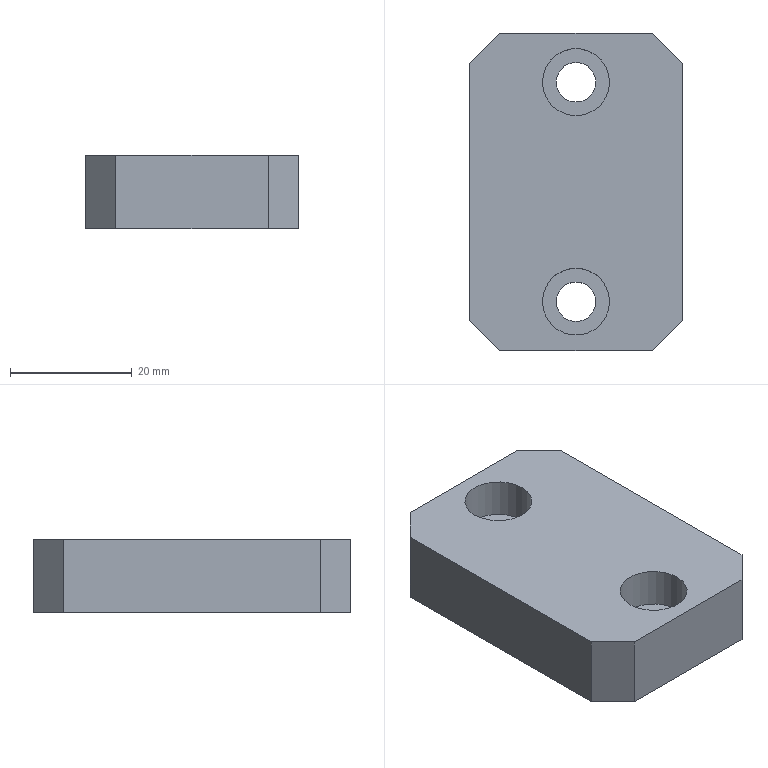Part | STEP file | lll_id314_x_t | 1 solid | 16 faces | box 35 x 52 x 12 mm | volume 19640 mm3 | plane 12 | cylinder 4 | commonest cylinder face diameters 6.5 x2 11 x2
STEP:
#1=CARTESIAN_POINT('',(76.553,9.,100.5));
#2=VERTEX_POINT('',#1);
#3=CARTESIAN_POINT('',(51.553,9.,100.5));
#4=VERTEX_POINT('',#3);
#5=CARTESIAN_POINT('',(-312.69,9.,100.5));
#6=DIRECTION('',(-1.,0.,0.));
#7=VECTOR('',#6,1.);
#8=LINE('',#5,#7);
#9=EDGE_CURVE('',#2,#4,#8,.T.);
#10=ORIENTED_EDGE('',*,*,#9,.T.);
#11=CARTESIAN_POINT('',(51.553,9.,88.5));
#12=VERTEX_POINT('',#11);
#13=CARTESIAN_POINT('',(51.553,9.,110.5));
#14=DIRECTION('',(0.,0.,1.));
#15=VECTOR('',#14,1.);
#16=LINE('',#13,#15);
#17=EDGE_CURVE('',#12,#4,#16,.T.);
#18=ORIENTED_EDGE('',*,*,#17,.F.);
#19=CARTESIAN_POINT('',(76.553,9.,88.5));
#20=VERTEX_POINT('',#19);
#21=CARTESIAN_POINT('',(64.053,9.,88.5));
#22=DIRECTION('',(1.,0.,0.));
#23=VECTOR('',#22,1.);
#24=LINE('',#21,#23);
#25=EDGE_CURVE('',#12,#20,#24,.T.);
#26=ORIENTED_EDGE('',*,*,#25,.T.);
#27=CARTESIAN_POINT('',(76.553,9.,88.5));
#28=DIRECTION('',(0.,0.,-1.));
#29=VECTOR('',#28,1.);
#30=LINE('',#27,#29);
#31=EDGE_CURVE('',#2,#20,#30,.T.);
#32=ORIENTED_EDGE('',*,*,#31,.F.);
#33=EDGE_LOOP('',(#10,#18,#26,#32));
#34=FACE_OUTER_BOUND('',#33,.T.);
#35=CARTESIAN_POINT('',(47.219,9.,110.5));
#36=DIRECTION('',(0.,-1.,0.));
#37=DIRECTION('',(0.,0.,1.));
#38=AXIS2_PLACEMENT_3D('',#35,#36,#37);
#39=PLANE('',#38);
#40=ADVANCED_FACE('',(#34),#39,.T.);
#41=CARTESIAN_POINT('',(81.553,56.,88.5));
#42=VERTEX_POINT('',#41);
#43=CARTESIAN_POINT('',(81.553,14.,88.5));
#44=VERTEX_POINT('',#43);
#45=CARTESIAN_POINT('',(81.553,34.,88.5));
#46=DIRECTION('',(0.,-1.,0.));
#47=VECTOR('',#46,1.);
#48=LINE('',#45,#47);
#49=EDGE_CURVE('',#42,#44,#48,.T.);
#50=ORIENTED_EDGE('',*,*,#49,.T.);
#51=CARTESIAN_POINT('',(86.803,19.25,88.5));
#52=DIRECTION('',(0.7071,0.7071,0.));
#53=VECTOR('',#52,1.);
#54=LINE('',#51,#53);
#55=EDGE_CURVE('',#20,#44,#54,.T.);
#56=ORIENTED_EDGE('',*,*,#55,.F.);
#57=ORIENTED_EDGE('',*,*,#25,.F.);
#58=CARTESIAN_POINT('',(46.553,14.,88.5));
#59=VERTEX_POINT('',#58);
#60=CARTESIAN_POINT('',(41.303,19.25,88.5));
#61=DIRECTION('',(0.7071,-0.7071,0.));
#62=VECTOR('',#61,1.);
#63=LINE('',#60,#62);
#64=EDGE_CURVE('',#59,#12,#63,.T.);
#65=ORIENTED_EDGE('',*,*,#64,.F.);
#66=CARTESIAN_POINT('',(46.553,56.,88.5));
#67=VERTEX_POINT('',#66);
#68=CARTESIAN_POINT('',(46.553,34.,88.5));
#69=DIRECTION('',(0.,-1.,0.));
#70=VECTOR('',#69,1.);
#71=LINE('',#68,#70);
#72=EDGE_CURVE('',#67,#59,#71,.T.);
#73=ORIENTED_EDGE('',*,*,#72,.F.);
#74=CARTESIAN_POINT('',(51.553,61.,88.5));
#75=VERTEX_POINT('',#74);
#76=CARTESIAN_POINT('',(44.303,53.75,88.5));
#77=DIRECTION('',(-0.7071,-0.7071,0.));
#78=VECTOR('',#77,1.);
#79=LINE('',#76,#78);
#80=EDGE_CURVE('',#75,#67,#79,.T.);
#81=ORIENTED_EDGE('',*,*,#80,.F.);
#82=CARTESIAN_POINT('',(76.553,61.,88.5));
#83=VERTEX_POINT('',#82);
#84=CARTESIAN_POINT('',(64.053,61.,88.5));
#85=DIRECTION('',(1.,0.,0.));
#86=VECTOR('',#85,1.);
#87=LINE('',#84,#86);
#88=EDGE_CURVE('',#75,#83,#87,.T.);
#89=ORIENTED_EDGE('',*,*,#88,.T.);
#90=CARTESIAN_POINT('',(83.803,53.75,88.5));
#91=DIRECTION('',(-0.7071,0.7071,0.));
#92=VECTOR('',#91,1.);
#93=LINE('',#90,#92);
#94=EDGE_CURVE('',#42,#83,#93,.T.);
#95=ORIENTED_EDGE('',*,*,#94,.F.);
#96=EDGE_LOOP('',(#50,#56,#57,#65,#73,#81,#89,#95));
#97=FACE_BOUND('',#96,.T.);
#98=CARTESIAN_POINT('',(67.303,17.,88.5));
#99=VERTEX_POINT('',#98);
#100=CARTESIAN_POINT('',(64.053,17.,88.5));
#101=DIRECTION('',(0.,0.,1.));
#102=DIRECTION('',(1.,0.,0.));
#103=AXIS2_PLACEMENT_3D('',#100,#101,#102);
#104=CIRCLE('',#103,3.25);
#105=EDGE_CURVE('',#99,#99,#104,.T.);
#106=ORIENTED_EDGE('',*,*,#105,.T.);
#107=EDGE_LOOP('',(#106));
#108=FACE_BOUND('',#107,.T.);
#109=CARTESIAN_POINT('',(67.303,53.,88.5));
#110=VERTEX_POINT('',#109);
#111=CARTESIAN_POINT('',(64.053,53.,88.5));
#112=DIRECTION('',(0.,0.,1.));
#113=DIRECTION('',(1.,0.,0.));
#114=AXIS2_PLACEMENT_3D('',#111,#112,#113);
#115=CIRCLE('',#114,3.25);
#116=EDGE_CURVE('',#110,#110,#115,.T.);
#117=ORIENTED_EDGE('',*,*,#116,.T.);
#118=EDGE_LOOP('',(#117));
#119=FACE_BOUND('',#118,.T.);
#120=CARTESIAN_POINT('',(64.053,34.,88.5));
#121=DIRECTION('',(0.,0.,-1.));
#122=DIRECTION('',(-1.,0.,0.));
#123=AXIS2_PLACEMENT_3D('',#120,#121,#122);
#124=PLANE('',#123);
#125=ADVANCED_FACE('',(#97,#108,#119),#124,.T.);
#126=CARTESIAN_POINT('',(76.553,61.,100.5));
#127=VERTEX_POINT('',#126);
#128=CARTESIAN_POINT('',(51.553,61.,100.5));
#129=VERTEX_POINT('',#128);
#130=CARTESIAN_POINT('',(-312.69,61.,100.5));
#131=DIRECTION('',(-1.,0.,0.));
#132=VECTOR('',#131,1.);
#133=LINE('',#130,#132);
#134=EDGE_CURVE('',#127,#129,#133,.T.);
#135=ORIENTED_EDGE('',*,*,#134,.T.);
#136=CARTESIAN_POINT('',(46.553,56.,100.5));
#137=VERTEX_POINT('',#136);
#138=CARTESIAN_POINT('',(-222.363,-212.917,100.5));
#139=DIRECTION('',(0.7071,0.7071,0.));
#140=VECTOR('',#139,1.);
#141=LINE('',#138,#140);
#142=EDGE_CURVE('',#137,#129,#141,.T.);
#143=ORIENTED_EDGE('',*,*,#142,.F.);
#144=CARTESIAN_POINT('',(46.553,14.,100.5));
#145=VERTEX_POINT('',#144);
#146=CARTESIAN_POINT('',(46.553,-122.59,100.5));
#147=DIRECTION('',(0.,1.,0.));
#148=VECTOR('',#147,1.);
#149=LINE('',#146,#148);
#150=EDGE_CURVE('',#145,#137,#149,.T.);
#151=ORIENTED_EDGE('',*,*,#150,.F.);
#152=CARTESIAN_POINT('',(-68.773,129.327,100.5));
#153=DIRECTION('',(-0.7071,0.7071,0.));
#154=VECTOR('',#153,1.);
#155=LINE('',#152,#154);
#156=EDGE_CURVE('',#4,#145,#155,.T.);
#157=ORIENTED_EDGE('',*,*,#156,.F.);
#158=ORIENTED_EDGE('',*,*,#9,.F.);
#159=CARTESIAN_POINT('',(81.553,14.,100.5));
#160=VERTEX_POINT('',#159);
#161=CARTESIAN_POINT('',(-179.863,-247.417,100.5));
#162=DIRECTION('',(-0.7071,-0.7071,0.));
#163=VECTOR('',#162,1.);
#164=LINE('',#161,#163);
#165=EDGE_CURVE('',#160,#2,#164,.T.);
#166=ORIENTED_EDGE('',*,*,#165,.F.);
#167=CARTESIAN_POINT('',(81.553,56.,100.5));
#168=VERTEX_POINT('',#167);
#169=CARTESIAN_POINT('',(81.553,-122.59,100.5));
#170=DIRECTION('',(0.,1.,0.));
#171=VECTOR('',#170,1.);
#172=LINE('',#169,#171);
#173=EDGE_CURVE('',#160,#168,#172,.T.);
#174=ORIENTED_EDGE('',*,*,#173,.T.);
#175=CARTESIAN_POINT('',(-26.273,163.827,100.5));
#176=DIRECTION('',(0.7071,-0.7071,0.));
#177=VECTOR('',#176,1.);
#178=LINE('',#175,#177);
#179=EDGE_CURVE('',#127,#168,#178,.T.);
#180=ORIENTED_EDGE('',*,*,#179,.F.);
#181=EDGE_LOOP('',(#135,#143,#151,#157,#158,#166,#174,#180));
#182=FACE_BOUND('',#181,.T.);
#183=CARTESIAN_POINT('',(58.553,17.,100.5));
#184=VERTEX_POINT('',#183);
#185=CARTESIAN_POINT('',(64.053,17.,100.5));
#186=DIRECTION('',(0.,0.,1.));
#187=DIRECTION('',(-1.,0.,0.));
#188=AXIS2_PLACEMENT_3D('',#185,#186,#187);
#189=CIRCLE('',#188,5.5);
#190=EDGE_CURVE('',#184,#184,#189,.T.);
#191=ORIENTED_EDGE('',*,*,#190,.F.);
#192=EDGE_LOOP('',(#191));
#193=FACE_BOUND('',#192,.T.);
#194=CARTESIAN_POINT('',(58.553,53.,100.5));
#195=VERTEX_POINT('',#194);
#196=CARTESIAN_POINT('',(64.053,53.,100.5));
#197=DIRECTION('',(0.,0.,-1.));
#198=DIRECTION('',(-1.,0.,0.));
#199=AXIS2_PLACEMENT_3D('',#196,#197,#198);
#200=CIRCLE('',#199,5.5);
#201=EDGE_CURVE('',#195,#195,#200,.T.);
#202=ORIENTED_EDGE('',*,*,#201,.T.);
#203=EDGE_LOOP('',(#202));
#204=FACE_BOUND('',#203,.T.);
#205=CARTESIAN_POINT('',(-312.69,-122.59,100.5));
#206=DIRECTION('',(0.,0.,-1.));
#207=DIRECTION('',(0.,-1.,0.));
#208=AXIS2_PLACEMENT_3D('',#205,#206,#207);
#209=PLANE('',#208);
#210=ADVANCED_FACE('',(#182,#193,#204),#209,.F.);
#211=ORIENTED_EDGE('',*,*,#88,.F.);
#212=CARTESIAN_POINT('',(51.553,61.,88.5));
#213=DIRECTION('',(0.,0.,-1.));
#214=VECTOR('',#213,1.);
#215=LINE('',#212,#214);
#216=EDGE_CURVE('',#129,#75,#215,.T.);
#217=ORIENTED_EDGE('',*,*,#216,.F.);
#218=ORIENTED_EDGE('',*,*,#134,.F.);
#219=CARTESIAN_POINT('',(76.553,61.,110.5));
#220=DIRECTION('',(0.,0.,1.));
#221=VECTOR('',#220,1.);
#222=LINE('',#219,#221);
#223=EDGE_CURVE('',#83,#127,#222,.T.);
#224=ORIENTED_EDGE('',*,*,#223,.F.);
#225=EDGE_LOOP('',(#211,#217,#218,#224));
#226=FACE_OUTER_BOUND('',#225,.T.);
#227=CARTESIAN_POINT('',(47.219,61.,110.5));
#228=DIRECTION('',(0.,-1.,0.));
#229=DIRECTION('',(0.,0.,1.));
#230=AXIS2_PLACEMENT_3D('',#227,#228,#229);
#231=PLANE('',#230);
#232=ADVANCED_FACE('',(#226),#231,.F.);
#233=ORIENTED_EDGE('',*,*,#105,.F.);
#234=EDGE_LOOP('',(#233));
#235=FACE_BOUND('',#234,.T.);
#236=CARTESIAN_POINT('',(60.803,17.,94.));
#237=VERTEX_POINT('',#236);
#238=CARTESIAN_POINT('',(64.053,17.,94.));
#239=DIRECTION('',(0.,0.,1.));
#240=DIRECTION('',(-1.,0.,0.));
#241=AXIS2_PLACEMENT_3D('',#238,#239,#240);
#242=CIRCLE('',#241,3.25);
#243=EDGE_CURVE('',#237,#237,#242,.T.);
#244=ORIENTED_EDGE('',*,*,#243,.T.);
#245=EDGE_LOOP('',(#244));
#246=FACE_BOUND('',#245,.T.);
#247=CARTESIAN_POINT('',(64.053,17.,-199.5));
#248=DIRECTION('',(0.,0.,-1.));
#249=DIRECTION('',(-1.,0.,0.));
#250=AXIS2_PLACEMENT_3D('',#247,#248,#249);
#251=CYLINDRICAL_SURFACE('',#250,3.25);
#252=ADVANCED_FACE('',(#235,#246),#251,.F.);
#253=ORIENTED_EDGE('',*,*,#243,.F.);
#254=EDGE_LOOP('',(#253));
#255=FACE_BOUND('',#254,.T.);
#256=CARTESIAN_POINT('',(58.553,17.,94.));
#257=VERTEX_POINT('',#256);
#258=CARTESIAN_POINT('',(64.053,17.,94.));
#259=DIRECTION('',(0.,0.,1.));
#260=DIRECTION('',(-1.,0.,0.));
#261=AXIS2_PLACEMENT_3D('',#258,#259,#260);
#262=CIRCLE('',#261,5.5);
#263=EDGE_CURVE('',#257,#257,#262,.T.);
#264=ORIENTED_EDGE('',*,*,#263,.T.);
#265=EDGE_LOOP('',(#264));
#266=FACE_BOUND('',#265,.T.);
#267=CARTESIAN_POINT('',(64.053,17.,94.));
#268=DIRECTION('',(0.,0.,-1.));
#269=DIRECTION('',(-1.,0.,0.));
#270=AXIS2_PLACEMENT_3D('',#267,#268,#269);
#271=PLANE('',#270);
#272=ADVANCED_FACE('',(#255,#266),#271,.F.);
#273=ORIENTED_EDGE('',*,*,#263,.F.);
#274=EDGE_LOOP('',(#273));
#275=FACE_BOUND('',#274,.T.);
#276=ORIENTED_EDGE('',*,*,#190,.T.);
#277=EDGE_LOOP('',(#276));
#278=FACE_BOUND('',#277,.T.);
#279=CARTESIAN_POINT('',(64.053,17.,100.5));
#280=DIRECTION('',(0.,0.,-1.));
#281=DIRECTION('',(-1.,0.,0.));
#282=AXIS2_PLACEMENT_3D('',#279,#280,#281);
#283=CYLINDRICAL_SURFACE('',#282,5.5);
#284=ADVANCED_FACE('',(#275,#278),#283,.F.);
#285=ORIENTED_EDGE('',*,*,#116,.F.);
#286=EDGE_LOOP('',(#285));
#287=FACE_BOUND('',#286,.T.);
#288=CARTESIAN_POINT('',(60.803,53.,94.));
#289=VERTEX_POINT('',#288);
#290=CARTESIAN_POINT('',(64.053,53.,94.));
#291=DIRECTION('',(0.,0.,-1.));
#292=DIRECTION('',(-1.,0.,0.));
#293=AXIS2_PLACEMENT_3D('',#290,#291,#292);
#294=CIRCLE('',#293,3.25);
#295=EDGE_CURVE('',#289,#289,#294,.T.);
#296=ORIENTED_EDGE('',*,*,#295,.F.);
#297=EDGE_LOOP('',(#296));
#298=FACE_BOUND('',#297,.T.);
#299=CARTESIAN_POINT('',(64.053,53.,-199.5));
#300=DIRECTION('',(0.,0.,-1.));
#301=DIRECTION('',(-1.,0.,0.));
#302=AXIS2_PLACEMENT_3D('',#299,#300,#301);
#303=CYLINDRICAL_SURFACE('',#302,3.25);
#304=ADVANCED_FACE('',(#287,#298),#303,.F.);
#305=ORIENTED_EDGE('',*,*,#295,.T.);
#306=EDGE_LOOP('',(#305));
#307=FACE_BOUND('',#306,.T.);
#308=CARTESIAN_POINT('',(58.553,53.,94.));
#309=VERTEX_POINT('',#308);
#310=CARTESIAN_POINT('',(64.053,53.,94.));
#311=DIRECTION('',(0.,0.,-1.));
#312=DIRECTION('',(-1.,0.,0.));
#313=AXIS2_PLACEMENT_3D('',#310,#311,#312);
#314=CIRCLE('',#313,5.5);
#315=EDGE_CURVE('',#309,#309,#314,.T.);
#316=ORIENTED_EDGE('',*,*,#315,.F.);
#317=EDGE_LOOP('',(#316));
#318=FACE_BOUND('',#317,.T.);
#319=CARTESIAN_POINT('',(64.053,53.,94.));
#320=DIRECTION('',(0.,0.,-1.));
#321=DIRECTION('',(-1.,0.,0.));
#322=AXIS2_PLACEMENT_3D('',#319,#320,#321);
#323=PLANE('',#322);
#324=ADVANCED_FACE('',(#307,#318),#323,.F.);
#325=ORIENTED_EDGE('',*,*,#315,.T.);
#326=EDGE_LOOP('',(#325));
#327=FACE_BOUND('',#326,.T.);
#328=ORIENTED_EDGE('',*,*,#201,.F.);
#329=EDGE_LOOP('',(#328));
#330=FACE_BOUND('',#329,.T.);
#331=CARTESIAN_POINT('',(64.053,53.,100.5));
#332=DIRECTION('',(0.,0.,-1.));
#333=DIRECTION('',(-1.,0.,0.));
#334=AXIS2_PLACEMENT_3D('',#331,#332,#333);
#335=CYLINDRICAL_SURFACE('',#334,5.5);
#336=ADVANCED_FACE('',(#327,#330),#335,.F.);
#337=ORIENTED_EDGE('',*,*,#72,.T.);
#338=CARTESIAN_POINT('',(46.553,14.,100.5));
#339=DIRECTION('',(0.,0.,-1.));
#340=VECTOR('',#339,1.);
#341=LINE('',#338,#340);
#342=EDGE_CURVE('',#145,#59,#341,.T.);
#343=ORIENTED_EDGE('',*,*,#342,.F.);
#344=ORIENTED_EDGE('',*,*,#150,.T.);
#345=CARTESIAN_POINT('',(46.553,56.,100.5));
#346=DIRECTION('',(0.,0.,1.));
#347=VECTOR('',#346,1.);
#348=LINE('',#345,#347);
#349=EDGE_CURVE('',#67,#137,#348,.T.);
#350=ORIENTED_EDGE('',*,*,#349,.F.);
#351=EDGE_LOOP('',(#337,#343,#344,#350));
#352=FACE_OUTER_BOUND('',#351,.T.);
#353=CARTESIAN_POINT('',(46.553,61.,100.5));
#354=DIRECTION('',(-1.,0.,0.));
#355=DIRECTION('',(0.,0.,-1.));
#356=AXIS2_PLACEMENT_3D('',#353,#354,#355);
#357=PLANE('',#356);
#358=ADVANCED_FACE('',(#352),#357,.T.);
#359=ORIENTED_EDGE('',*,*,#173,.F.);
#360=CARTESIAN_POINT('',(81.553,14.,100.5));
#361=DIRECTION('',(0.,0.,1.));
#362=VECTOR('',#361,1.);
#363=LINE('',#360,#362);
#364=EDGE_CURVE('',#44,#160,#363,.T.);
#365=ORIENTED_EDGE('',*,*,#364,.F.);
#366=ORIENTED_EDGE('',*,*,#49,.F.);
#367=CARTESIAN_POINT('',(81.553,56.,100.5));
#368=DIRECTION('',(0.,0.,-1.));
#369=VECTOR('',#368,1.);
#370=LINE('',#367,#369);
#371=EDGE_CURVE('',#168,#42,#370,.T.);
#372=ORIENTED_EDGE('',*,*,#371,.F.);
#373=EDGE_LOOP('',(#359,#365,#366,#372));
#374=FACE_OUTER_BOUND('',#373,.T.);
#375=CARTESIAN_POINT('',(81.553,61.,100.5));
#376=DIRECTION('',(-1.,0.,0.));
#377=DIRECTION('',(0.,0.,-1.));
#378=AXIS2_PLACEMENT_3D('',#375,#376,#377);
#379=PLANE('',#378);
#380=ADVANCED_FACE('',(#374),#379,.F.);
#381=ORIENTED_EDGE('',*,*,#94,.T.);
#382=ORIENTED_EDGE('',*,*,#223,.T.);
#383=ORIENTED_EDGE('',*,*,#179,.T.);
#384=ORIENTED_EDGE('',*,*,#371,.T.);
#385=EDGE_LOOP('',(#381,#382,#383,#384));
#386=FACE_OUTER_BOUND('',#385,.T.);
#387=CARTESIAN_POINT('',(76.553,61.,110.5));
#388=DIRECTION('',(-0.7071,-0.7071,0.));
#389=DIRECTION('',(-0.7071,0.7071,0.));
#390=AXIS2_PLACEMENT_3D('',#387,#388,#389);
#391=PLANE('',#390);
#392=ADVANCED_FACE('',(#386),#391,.F.);
#393=ORIENTED_EDGE('',*,*,#80,.T.);
#394=ORIENTED_EDGE('',*,*,#349,.T.);
#395=ORIENTED_EDGE('',*,*,#142,.T.);
#396=ORIENTED_EDGE('',*,*,#216,.T.);
#397=EDGE_LOOP('',(#393,#394,#395,#396));
#398=FACE_OUTER_BOUND('',#397,.T.);
#399=CARTESIAN_POINT('',(46.553,56.,100.5));
#400=DIRECTION('',(-0.7071,0.7071,0.));
#401=DIRECTION('',(0.7071,0.7071,0.));
#402=AXIS2_PLACEMENT_3D('',#399,#400,#401);
#403=PLANE('',#402);
#404=ADVANCED_FACE('',(#398),#403,.T.);
#405=ORIENTED_EDGE('',*,*,#55,.T.);
#406=ORIENTED_EDGE('',*,*,#364,.T.);
#407=ORIENTED_EDGE('',*,*,#165,.T.);
#408=ORIENTED_EDGE('',*,*,#31,.T.);
#409=EDGE_LOOP('',(#405,#406,#407,#408));
#410=FACE_OUTER_BOUND('',#409,.T.);
#411=CARTESIAN_POINT('',(81.553,14.,100.5));
#412=DIRECTION('',(0.7071,-0.7071,0.));
#413=DIRECTION('',(-0.7071,-0.7071,0.));
#414=AXIS2_PLACEMENT_3D('',#411,#412,#413);
#415=PLANE('',#414);
#416=ADVANCED_FACE('',(#410),#415,.T.);
#417=ORIENTED_EDGE('',*,*,#64,.T.);
#418=ORIENTED_EDGE('',*,*,#17,.T.);
#419=ORIENTED_EDGE('',*,*,#156,.T.);
#420=ORIENTED_EDGE('',*,*,#342,.T.);
#421=EDGE_LOOP('',(#417,#418,#419,#420));
#422=FACE_OUTER_BOUND('',#421,.T.);
#423=CARTESIAN_POINT('',(51.553,9.,110.5));
#424=DIRECTION('',(0.7071,0.7071,0.));
#425=DIRECTION('',(0.7071,-0.7071,0.));
#426=AXIS2_PLACEMENT_3D('',#423,#424,#425);
#427=PLANE('',#426);
#428=ADVANCED_FACE('',(#422),#427,.F.);
#429=CLOSED_SHELL('',(#40,#125,#210,#232,#252,#272,#284,#304,#324,#336,#358,#380,#392,#404,#416,#428));
#430=MANIFOLD_SOLID_BREP('',#429);
#431=(LENGTH_UNIT()NAMED_UNIT(*)SI_UNIT(.MILLI.,.METRE.));
#432=UNCERTAINTY_MEASURE_WITH_UNIT(LENGTH_MEASURE(0.00002),#431,'','');
#433=(NAMED_UNIT(*)PLANE_ANGLE_UNIT()SI_UNIT($,.RADIAN.));
#434=PLANE_ANGLE_MEASURE_WITH_UNIT(PLANE_ANGLE_MEASURE(0.01745),#433);
#435=DIMENSIONAL_EXPONENTS(0.,0.,0.,0.,0.,0.,0.);
#436=(CONVERSION_BASED_UNIT('DEGREE',#434)NAMED_UNIT(#435)PLANE_ANGLE_UNIT());
#437=(NAMED_UNIT(*)SI_UNIT($,.STERADIAN.)SOLID_ANGLE_UNIT());
#438=(GEOMETRIC_REPRESENTATION_CONTEXT(3)GLOBAL_UNCERTAINTY_ASSIGNED_CONTEXT((#432))GLOBAL_UNIT_ASSIGNED_CONTEXT((#431,#436,#437))REPRESENTATION_CONTEXT('',''));
#439=ADVANCED_BREP_SHAPE_REPRESENTATION('',(#430),#438);